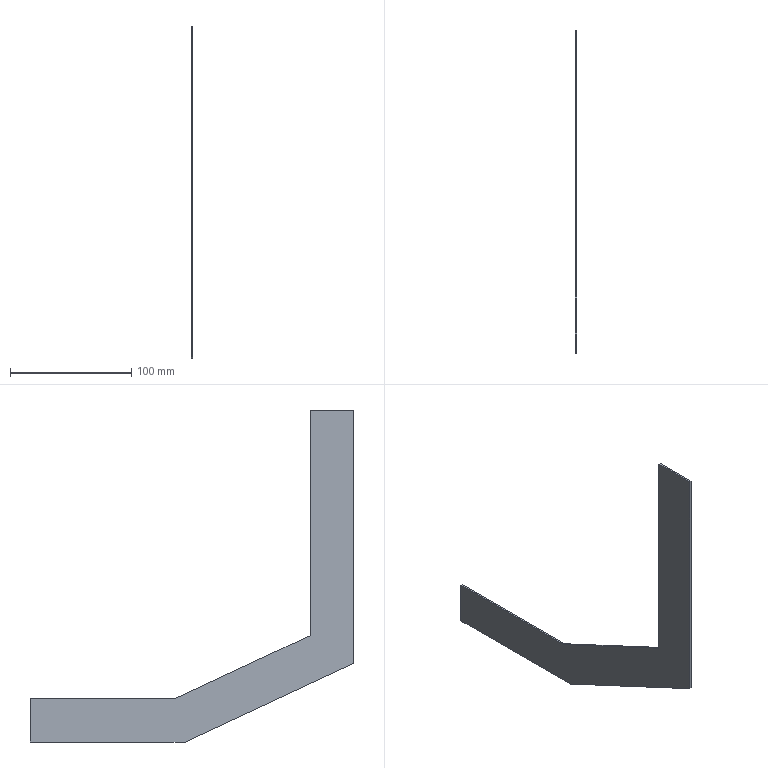Part | NX | features solid 2 | 1 solid | 10 faces | box 1.5 x 267 x 274 mm | volume 24816 mm3 | plane 10
STEP:
#1=CARTESIAN_POINT('',(1142.,-1540.,465.));
#2=VERTEX_POINT('',#1);
#3=CARTESIAN_POINT('',(1142.,-1540.,278.859));
#4=VERTEX_POINT('',#3);
#5=CARTESIAN_POINT('',(1142.,-1540.,465.));
#6=DIRECTION('',(0.,0.,-1.));
#7=VECTOR('',#6,1000.);
#8=LINE('',#5,#7);
#9=EDGE_CURVE('',#2,#4,#8,.T.);
#10=ORIENTED_EDGE('',*,*,#9,.F.);
#11=CARTESIAN_POINT('',(1142.,-1576.,465.));
#12=VERTEX_POINT('',#11);
#13=CARTESIAN_POINT('',(1142.,-1576.,465.));
#14=DIRECTION('',(0.,1.,0.));
#15=VECTOR('',#14,1000.);
#16=LINE('',#13,#15);
#17=EDGE_CURVE('',#12,#2,#16,.T.);
#18=ORIENTED_EDGE('',*,*,#17,.F.);
#19=CARTESIAN_POINT('',(1142.,-1576.,255.924));
#20=VERTEX_POINT('',#19);
#21=CARTESIAN_POINT('',(1142.,-1576.,465.));
#22=DIRECTION('',(0.,0.,1.));
#23=VECTOR('',#22,1000.);
#24=LINE('',#21,#23);
#25=EDGE_CURVE('',#20,#12,#24,.T.);
#26=ORIENTED_EDGE('',*,*,#25,.F.);
#27=CARTESIAN_POINT('',(1142.,-1436.769,191.));
#28=VERTEX_POINT('',#27);
#29=CARTESIAN_POINT('',(1142.,-1576.,255.924));
#30=DIRECTION('',(0.,-0.9063,0.4226));
#31=VECTOR('',#30,1000.);
#32=LINE('',#29,#31);
#33=EDGE_CURVE('',#28,#20,#32,.T.);
#34=ORIENTED_EDGE('',*,*,#33,.F.);
#35=CARTESIAN_POINT('',(1142.,-1309.,191.));
#36=VERTEX_POINT('',#35);
#37=CARTESIAN_POINT('',(1142.,-1436.769,191.));
#38=DIRECTION('',(0.,-1.,0.));
#39=VECTOR('',#38,1000.);
#40=LINE('',#37,#39);
#41=EDGE_CURVE('',#36,#28,#40,.T.);
#42=ORIENTED_EDGE('',*,*,#41,.F.);
#43=CARTESIAN_POINT('',(1142.,-1309.,227.));
#44=VERTEX_POINT('',#43);
#45=CARTESIAN_POINT('',(1142.,-1309.,191.));
#46=DIRECTION('',(0.,0.,-1.));
#47=VECTOR('',#46,1000.);
#48=LINE('',#45,#47);
#49=EDGE_CURVE('',#44,#36,#48,.T.);
#50=ORIENTED_EDGE('',*,*,#49,.F.);
#51=CARTESIAN_POINT('',(1142.,-1428.788,227.));
#52=VERTEX_POINT('',#51);
#53=CARTESIAN_POINT('',(1142.,-1428.788,227.));
#54=DIRECTION('',(0.,1.,0.));
#55=VECTOR('',#54,1000.);
#56=LINE('',#53,#55);
#57=EDGE_CURVE('',#52,#44,#56,.T.);
#58=ORIENTED_EDGE('',*,*,#57,.F.);
#59=CARTESIAN_POINT('',(1142.,-1540.,278.859));
#60=DIRECTION('',(0.,0.9063,-0.4226));
#61=VECTOR('',#60,1000.);
#62=LINE('',#59,#61);
#63=EDGE_CURVE('',#4,#52,#62,.T.);
#64=ORIENTED_EDGE('',*,*,#63,.F.);
#65=EDGE_LOOP('',(#10,#18,#26,#34,#42,#50,#58,#64));
#66=FACE_BOUND('',#65,.T.);
#67=CARTESIAN_POINT('',(1142.,0.,0.));
#68=DIRECTION('',(1.,0.,0.));
#69=DIRECTION('',(0.,0.,-1.));
#70=AXIS2_PLACEMENT_3D('',#67,#68,#69);
#71=PLANE('',#70);
#72=ADVANCED_FACE('',(#66),#71,.T.);
#73=CARTESIAN_POINT('',(1140.5,-1540.,465.));
#74=VERTEX_POINT('',#73);
#75=CARTESIAN_POINT('',(1140.5,-1540.,278.859));
#76=VERTEX_POINT('',#75);
#77=CARTESIAN_POINT('',(1140.5,-1540.,465.));
#78=DIRECTION('',(0.,0.,-1.));
#79=VECTOR('',#78,1000.);
#80=LINE('',#77,#79);
#81=EDGE_CURVE('',#74,#76,#80,.T.);
#82=ORIENTED_EDGE('',*,*,#81,.T.);
#83=CARTESIAN_POINT('',(1140.5,-1428.788,227.));
#84=VERTEX_POINT('',#83);
#85=CARTESIAN_POINT('',(1140.5,-1540.,278.859));
#86=DIRECTION('',(0.,0.9063,-0.4226));
#87=VECTOR('',#86,1000.);
#88=LINE('',#85,#87);
#89=EDGE_CURVE('',#76,#84,#88,.T.);
#90=ORIENTED_EDGE('',*,*,#89,.T.);
#91=CARTESIAN_POINT('',(1140.5,-1309.,227.));
#92=VERTEX_POINT('',#91);
#93=CARTESIAN_POINT('',(1140.5,-1428.788,227.));
#94=DIRECTION('',(0.,1.,0.));
#95=VECTOR('',#94,1000.);
#96=LINE('',#93,#95);
#97=EDGE_CURVE('',#84,#92,#96,.T.);
#98=ORIENTED_EDGE('',*,*,#97,.T.);
#99=CARTESIAN_POINT('',(1140.5,-1309.,191.));
#100=VERTEX_POINT('',#99);
#101=CARTESIAN_POINT('',(1140.5,-1309.,191.));
#102=DIRECTION('',(0.,0.,-1.));
#103=VECTOR('',#102,1000.);
#104=LINE('',#101,#103);
#105=EDGE_CURVE('',#92,#100,#104,.T.);
#106=ORIENTED_EDGE('',*,*,#105,.T.);
#107=CARTESIAN_POINT('',(1140.5,-1436.769,191.));
#108=VERTEX_POINT('',#107);
#109=CARTESIAN_POINT('',(1140.5,-1436.769,191.));
#110=DIRECTION('',(0.,-1.,0.));
#111=VECTOR('',#110,1000.);
#112=LINE('',#109,#111);
#113=EDGE_CURVE('',#100,#108,#112,.T.);
#114=ORIENTED_EDGE('',*,*,#113,.T.);
#115=CARTESIAN_POINT('',(1140.5,-1576.,255.924));
#116=VERTEX_POINT('',#115);
#117=CARTESIAN_POINT('',(1140.5,-1576.,255.924));
#118=DIRECTION('',(0.,-0.9063,0.4226));
#119=VECTOR('',#118,1000.);
#120=LINE('',#117,#119);
#121=EDGE_CURVE('',#108,#116,#120,.T.);
#122=ORIENTED_EDGE('',*,*,#121,.T.);
#123=CARTESIAN_POINT('',(1140.5,-1576.,465.));
#124=VERTEX_POINT('',#123);
#125=CARTESIAN_POINT('',(1140.5,-1576.,465.));
#126=DIRECTION('',(0.,0.,1.));
#127=VECTOR('',#126,1000.);
#128=LINE('',#125,#127);
#129=EDGE_CURVE('',#116,#124,#128,.T.);
#130=ORIENTED_EDGE('',*,*,#129,.T.);
#131=CARTESIAN_POINT('',(1140.5,-1576.,465.));
#132=DIRECTION('',(0.,1.,0.));
#133=VECTOR('',#132,1000.);
#134=LINE('',#131,#133);
#135=EDGE_CURVE('',#124,#74,#134,.T.);
#136=ORIENTED_EDGE('',*,*,#135,.T.);
#137=EDGE_LOOP('',(#82,#90,#98,#106,#114,#122,#130,#136));
#138=FACE_BOUND('',#137,.T.);
#139=CARTESIAN_POINT('',(1140.5,0.,0.));
#140=DIRECTION('',(1.,0.,0.));
#141=DIRECTION('',(0.,0.,-1.));
#142=AXIS2_PLACEMENT_3D('',#139,#140,#141);
#143=PLANE('',#142);
#144=ADVANCED_FACE('',(#138),#143,.F.);
#145=ORIENTED_EDGE('',*,*,#17,.T.);
#146=CARTESIAN_POINT('',(1140.5,-1540.,465.));
#147=DIRECTION('',(1.,0.,0.));
#148=VECTOR('',#147,1000.);
#149=LINE('',#146,#148);
#150=EDGE_CURVE('',#74,#2,#149,.T.);
#151=ORIENTED_EDGE('',*,*,#150,.F.);
#152=ORIENTED_EDGE('',*,*,#135,.F.);
#153=CARTESIAN_POINT('',(1140.5,-1576.,465.));
#154=DIRECTION('',(1.,0.,0.));
#155=VECTOR('',#154,1000.);
#156=LINE('',#153,#155);
#157=EDGE_CURVE('',#124,#12,#156,.T.);
#158=ORIENTED_EDGE('',*,*,#157,.T.);
#159=EDGE_LOOP('',(#145,#151,#152,#158));
#160=FACE_BOUND('',#159,.T.);
#161=CARTESIAN_POINT('',(1140.5,-1576.,465.));
#162=DIRECTION('',(0.,0.,-1.));
#163=DIRECTION('',(-1.,0.,0.));
#164=AXIS2_PLACEMENT_3D('',#161,#162,#163);
#165=PLANE('',#164);
#166=ADVANCED_FACE('',(#160),#165,.F.);
#167=ORIENTED_EDGE('',*,*,#25,.T.);
#168=ORIENTED_EDGE('',*,*,#157,.F.);
#169=ORIENTED_EDGE('',*,*,#129,.F.);
#170=CARTESIAN_POINT('',(1140.5,-1576.,255.924));
#171=DIRECTION('',(1.,0.,0.));
#172=VECTOR('',#171,1000.);
#173=LINE('',#170,#172);
#174=EDGE_CURVE('',#116,#20,#173,.T.);
#175=ORIENTED_EDGE('',*,*,#174,.T.);
#176=EDGE_LOOP('',(#167,#168,#169,#175));
#177=FACE_BOUND('',#176,.T.);
#178=CARTESIAN_POINT('',(1140.5,-1576.,465.));
#179=DIRECTION('',(0.,1.,0.));
#180=DIRECTION('',(0.,0.,-1.));
#181=AXIS2_PLACEMENT_3D('',#178,#179,#180);
#182=PLANE('',#181);
#183=ADVANCED_FACE('',(#177),#182,.F.);
#184=ORIENTED_EDGE('',*,*,#33,.T.);
#185=ORIENTED_EDGE('',*,*,#174,.F.);
#186=ORIENTED_EDGE('',*,*,#121,.F.);
#187=CARTESIAN_POINT('',(1140.5,-1436.769,191.));
#188=DIRECTION('',(1.,0.,0.));
#189=VECTOR('',#188,1000.);
#190=LINE('',#187,#189);
#191=EDGE_CURVE('',#108,#28,#190,.T.);
#192=ORIENTED_EDGE('',*,*,#191,.T.);
#193=EDGE_LOOP('',(#184,#185,#186,#192));
#194=FACE_BOUND('',#193,.T.);
#195=CARTESIAN_POINT('',(1140.5,-1576.,255.924));
#196=DIRECTION('',(0.,0.4226,0.9063));
#197=DIRECTION('',(1.,0.,0.));
#198=AXIS2_PLACEMENT_3D('',#195,#196,#197);
#199=PLANE('',#198);
#200=ADVANCED_FACE('',(#194),#199,.F.);
#201=ORIENTED_EDGE('',*,*,#41,.T.);
#202=ORIENTED_EDGE('',*,*,#191,.F.);
#203=ORIENTED_EDGE('',*,*,#113,.F.);
#204=CARTESIAN_POINT('',(1140.5,-1309.,191.));
#205=DIRECTION('',(1.,0.,0.));
#206=VECTOR('',#205,1000.);
#207=LINE('',#204,#206);
#208=EDGE_CURVE('',#100,#36,#207,.T.);
#209=ORIENTED_EDGE('',*,*,#208,.T.);
#210=EDGE_LOOP('',(#201,#202,#203,#209));
#211=FACE_BOUND('',#210,.T.);
#212=CARTESIAN_POINT('',(1140.5,-1436.769,191.));
#213=DIRECTION('',(0.,0.,1.));
#214=DIRECTION('',(0.,-1.,0.));
#215=AXIS2_PLACEMENT_3D('',#212,#213,#214);
#216=PLANE('',#215);
#217=ADVANCED_FACE('',(#211),#216,.F.);
#218=ORIENTED_EDGE('',*,*,#49,.T.);
#219=ORIENTED_EDGE('',*,*,#208,.F.);
#220=ORIENTED_EDGE('',*,*,#105,.F.);
#221=CARTESIAN_POINT('',(1140.5,-1309.,227.));
#222=DIRECTION('',(1.,0.,0.));
#223=VECTOR('',#222,1000.);
#224=LINE('',#221,#223);
#225=EDGE_CURVE('',#92,#44,#224,.T.);
#226=ORIENTED_EDGE('',*,*,#225,.T.);
#227=EDGE_LOOP('',(#218,#219,#220,#226));
#228=FACE_BOUND('',#227,.T.);
#229=CARTESIAN_POINT('',(1140.5,-1309.,191.));
#230=DIRECTION('',(0.,-1.,0.));
#231=DIRECTION('',(-1.,0.,0.));
#232=AXIS2_PLACEMENT_3D('',#229,#230,#231);
#233=PLANE('',#232);
#234=ADVANCED_FACE('',(#228),#233,.F.);
#235=ORIENTED_EDGE('',*,*,#57,.T.);
#236=ORIENTED_EDGE('',*,*,#225,.F.);
#237=ORIENTED_EDGE('',*,*,#97,.F.);
#238=CARTESIAN_POINT('',(1140.5,-1428.788,227.));
#239=DIRECTION('',(1.,0.,0.));
#240=VECTOR('',#239,1000.);
#241=LINE('',#238,#240);
#242=EDGE_CURVE('',#84,#52,#241,.T.);
#243=ORIENTED_EDGE('',*,*,#242,.T.);
#244=EDGE_LOOP('',(#235,#236,#237,#243));
#245=FACE_BOUND('',#244,.T.);
#246=CARTESIAN_POINT('',(1140.5,-1428.788,227.));
#247=DIRECTION('',(0.,0.,-1.));
#248=DIRECTION('',(0.,-1.,0.));
#249=AXIS2_PLACEMENT_3D('',#246,#247,#248);
#250=PLANE('',#249);
#251=ADVANCED_FACE('',(#245),#250,.F.);
#252=ORIENTED_EDGE('',*,*,#63,.T.);
#253=ORIENTED_EDGE('',*,*,#242,.F.);
#254=ORIENTED_EDGE('',*,*,#89,.F.);
#255=CARTESIAN_POINT('',(1140.5,-1540.,278.859));
#256=DIRECTION('',(1.,0.,0.));
#257=VECTOR('',#256,1000.);
#258=LINE('',#255,#257);
#259=EDGE_CURVE('',#76,#4,#258,.T.);
#260=ORIENTED_EDGE('',*,*,#259,.T.);
#261=EDGE_LOOP('',(#252,#253,#254,#260));
#262=FACE_BOUND('',#261,.T.);
#263=CARTESIAN_POINT('',(1140.5,-1540.,278.859));
#264=DIRECTION('',(0.,-0.4226,-0.9063));
#265=DIRECTION('',(0.,-0.9063,0.4226));
#266=AXIS2_PLACEMENT_3D('',#263,#264,#265);
#267=PLANE('',#266);
#268=ADVANCED_FACE('',(#262),#267,.F.);
#269=ORIENTED_EDGE('',*,*,#9,.T.);
#270=ORIENTED_EDGE('',*,*,#259,.F.);
#271=ORIENTED_EDGE('',*,*,#81,.F.);
#272=ORIENTED_EDGE('',*,*,#150,.T.);
#273=EDGE_LOOP('',(#269,#270,#271,#272));
#274=FACE_BOUND('',#273,.T.);
#275=CARTESIAN_POINT('',(1140.5,-1540.,465.));
#276=DIRECTION('',(0.,-1.,0.));
#277=DIRECTION('',(-1.,0.,0.));
#278=AXIS2_PLACEMENT_3D('',#275,#276,#277);
#279=PLANE('',#278);
#280=ADVANCED_FACE('',(#274),#279,.F.);
#281=CLOSED_SHELL('',(#72,#144,#166,#183,#200,#217,#234,#251,#268,#280));
#282=MANIFOLD_SOLID_BREP('',#281);
#283=(LENGTH_UNIT()NAMED_UNIT(*)SI_UNIT(.MILLI.,.METRE.));
#284=UNCERTAINTY_MEASURE_WITH_UNIT(LENGTH_MEASURE(0.00001),#283,'','');
#285=(NAMED_UNIT(*)PLANE_ANGLE_UNIT()SI_UNIT($,.RADIAN.));
#286=(NAMED_UNIT(*)SI_UNIT($,.STERADIAN.)SOLID_ANGLE_UNIT());
#287=(GEOMETRIC_REPRESENTATION_CONTEXT(3)GLOBAL_UNCERTAINTY_ASSIGNED_CONTEXT((#284))GLOBAL_UNIT_ASSIGNED_CONTEXT((#283,#285,#286))REPRESENTATION_CONTEXT('',''));
#288=ADVANCED_BREP_SHAPE_REPRESENTATION('',(#282),#287);